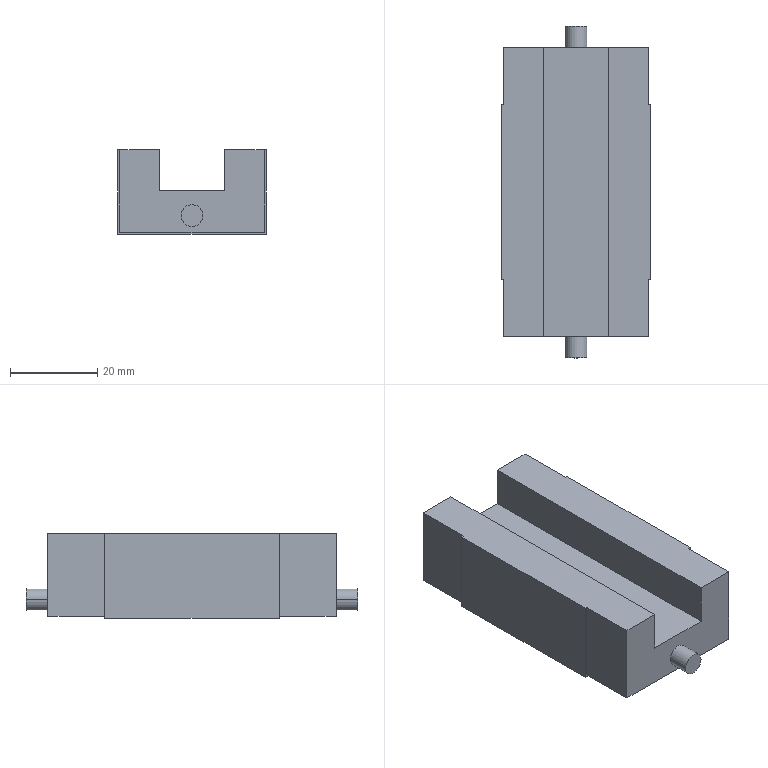Part | NX | 1 solid | 40 faces | box 34 x 76 x 19.4 mm | volume 33253 mm3 | plane 20 | cylinder 12 | cone 8 | commonest cylinder face diameters 3.3 x8 5 x4
STEP:
#1=CARTESIAN_POINT('',(33.5,0.,-18.9));
#2=VERTEX_POINT('',#1);
#3=CARTESIAN_POINT('',(33.5,0.,0.));
#4=VERTEX_POINT('',#3);
#5=CARTESIAN_POINT('',(33.5,0.,-18.9));
#6=DIRECTION('',(0.,0.,1.));
#7=VECTOR('',#6,1000.);
#8=LINE('',#5,#7);
#9=EDGE_CURVE('',#2,#4,#8,.T.);
#10=ORIENTED_EDGE('',*,*,#9,.T.);
#11=CARTESIAN_POINT('',(24.5,0.,0.));
#12=VERTEX_POINT('',#11);
#13=CARTESIAN_POINT('',(33.5,0.,0.));
#14=DIRECTION('',(-1.,0.,0.));
#15=VECTOR('',#14,1000.);
#16=LINE('',#13,#15);
#17=EDGE_CURVE('',#4,#12,#16,.T.);
#18=ORIENTED_EDGE('',*,*,#17,.T.);
#19=CARTESIAN_POINT('',(24.5,0.,-9.4));
#20=VERTEX_POINT('',#19);
#21=CARTESIAN_POINT('',(24.5,0.,0.));
#22=DIRECTION('',(0.,0.,-1.));
#23=VECTOR('',#22,1000.);
#24=LINE('',#21,#23);
#25=EDGE_CURVE('',#12,#20,#24,.T.);
#26=ORIENTED_EDGE('',*,*,#25,.T.);
#27=CARTESIAN_POINT('',(9.5,0.,-9.4));
#28=VERTEX_POINT('',#27);
#29=CARTESIAN_POINT('',(24.5,0.,-9.4));
#30=DIRECTION('',(-1.,0.,0.));
#31=VECTOR('',#30,1000.);
#32=LINE('',#29,#31);
#33=EDGE_CURVE('',#20,#28,#32,.T.);
#34=ORIENTED_EDGE('',*,*,#33,.T.);
#35=CARTESIAN_POINT('',(9.5,0.,0.));
#36=VERTEX_POINT('',#35);
#37=CARTESIAN_POINT('',(9.5,0.,-9.4));
#38=DIRECTION('',(0.,0.,1.));
#39=VECTOR('',#38,1000.);
#40=LINE('',#37,#39);
#41=EDGE_CURVE('',#28,#36,#40,.T.);
#42=ORIENTED_EDGE('',*,*,#41,.T.);
#43=CARTESIAN_POINT('',(0.5,0.,0.));
#44=VERTEX_POINT('',#43);
#45=CARTESIAN_POINT('',(9.5,0.,0.));
#46=DIRECTION('',(-1.,0.,0.));
#47=VECTOR('',#46,1000.);
#48=LINE('',#45,#47);
#49=EDGE_CURVE('',#36,#44,#48,.T.);
#50=ORIENTED_EDGE('',*,*,#49,.T.);
#51=CARTESIAN_POINT('',(0.5,0.,-18.9));
#52=VERTEX_POINT('',#51);
#53=CARTESIAN_POINT('',(0.5,0.,-18.9));
#54=DIRECTION('',(0.,0.,1.));
#55=VECTOR('',#54,1000.);
#56=LINE('',#53,#55);
#57=EDGE_CURVE('',#52,#44,#56,.T.);
#58=ORIENTED_EDGE('',*,*,#57,.F.);
#59=CARTESIAN_POINT('',(33.5,0.,-18.9));
#60=DIRECTION('',(-1.,0.,0.));
#61=VECTOR('',#60,1000.);
#62=LINE('',#59,#61);
#63=EDGE_CURVE('',#2,#52,#62,.T.);
#64=ORIENTED_EDGE('',*,*,#63,.F.);
#65=EDGE_LOOP('',(#10,#18,#26,#34,#42,#50,#58,#64));
#66=FACE_BOUND('',#65,.T.);
#67=CARTESIAN_POINT('',(19.5,0.,-15.1));
#68=VERTEX_POINT('',#67);
#69=CARTESIAN_POINT('',(14.5,0.,-15.1));
#70=VERTEX_POINT('',#69);
#71=CARTESIAN_POINT('',(17.,0.,-15.1));
#72=DIRECTION('',(0.,-1.,0.));
#73=DIRECTION('',(1.,0.,0.));
#74=AXIS2_PLACEMENT_3D('',#71,#72,#73);
#75=CIRCLE('',#74,2.5);
#76=EDGE_CURVE('',#68,#70,#75,.T.);
#77=ORIENTED_EDGE('',*,*,#76,.F.);
#78=CARTESIAN_POINT('',(17.,0.,-15.1));
#79=DIRECTION('',(0.,-1.,0.));
#80=DIRECTION('',(1.,0.,0.));
#81=AXIS2_PLACEMENT_3D('',#78,#79,#80);
#82=CIRCLE('',#81,2.5);
#83=EDGE_CURVE('',#70,#68,#82,.T.);
#84=ORIENTED_EDGE('',*,*,#83,.F.);
#85=EDGE_LOOP('',(#77,#84));
#86=FACE_BOUND('',#85,.T.);
#87=CARTESIAN_POINT('',(0.,0.,0.));
#88=DIRECTION('',(0.,1.,0.));
#89=DIRECTION('',(1.,0.,0.));
#90=AXIS2_PLACEMENT_3D('',#87,#88,#89);
#91=PLANE('',#90);
#92=ADVANCED_FACE('',(#66,#86),#91,.F.);
#93=ORIENTED_EDGE('',*,*,#9,.F.);
#94=CARTESIAN_POINT('',(33.5,13.,-18.9));
#95=VERTEX_POINT('',#94);
#96=CARTESIAN_POINT('',(33.5,0.,-18.9));
#97=DIRECTION('',(0.,1.,0.));
#98=VECTOR('',#97,1000.);
#99=LINE('',#96,#98);
#100=EDGE_CURVE('',#2,#95,#99,.T.);
#101=ORIENTED_EDGE('',*,*,#100,.T.);
#102=CARTESIAN_POINT('',(33.5,13.,0.));
#103=VERTEX_POINT('',#102);
#104=CARTESIAN_POINT('',(33.5,13.,0.));
#105=DIRECTION('',(0.,0.,-1.));
#106=VECTOR('',#105,1000.);
#107=LINE('',#104,#106);
#108=EDGE_CURVE('',#103,#95,#107,.T.);
#109=ORIENTED_EDGE('',*,*,#108,.F.);
#110=CARTESIAN_POINT('',(33.5,13.,0.));
#111=DIRECTION('',(0.,-1.,0.));
#112=VECTOR('',#111,1000.);
#113=LINE('',#110,#112);
#114=EDGE_CURVE('',#103,#4,#113,.T.);
#115=ORIENTED_EDGE('',*,*,#114,.T.);
#116=EDGE_LOOP('',(#93,#101,#109,#115));
#117=FACE_BOUND('',#116,.T.);
#118=CARTESIAN_POINT('',(33.5,0.,-18.9));
#119=DIRECTION('',(-1.,0.,0.));
#120=DIRECTION('',(0.,0.,1.));
#121=AXIS2_PLACEMENT_3D('',#118,#119,#120);
#122=PLANE('',#121);
#123=ADVANCED_FACE('',(#117),#122,.F.);
#124=CARTESIAN_POINT('',(33.5,53.,0.));
#125=VERTEX_POINT('',#124);
#126=CARTESIAN_POINT('',(34.,53.,0.));
#127=VERTEX_POINT('',#126);
#128=CARTESIAN_POINT('',(33.5,53.,0.));
#129=DIRECTION('',(1.,0.,0.));
#130=VECTOR('',#129,1000.);
#131=LINE('',#128,#130);
#132=EDGE_CURVE('',#125,#127,#131,.T.);
#133=ORIENTED_EDGE('',*,*,#132,.F.);
#134=CARTESIAN_POINT('',(33.5,66.,0.));
#135=VERTEX_POINT('',#134);
#136=CARTESIAN_POINT('',(33.5,53.,0.));
#137=DIRECTION('',(0.,1.,0.));
#138=VECTOR('',#137,1000.);
#139=LINE('',#136,#138);
#140=EDGE_CURVE('',#125,#135,#139,.T.);
#141=ORIENTED_EDGE('',*,*,#140,.T.);
#142=CARTESIAN_POINT('',(24.5,66.,0.));
#143=VERTEX_POINT('',#142);
#144=CARTESIAN_POINT('',(33.5,66.,0.));
#145=DIRECTION('',(-1.,0.,0.));
#146=VECTOR('',#145,1000.);
#147=LINE('',#144,#146);
#148=EDGE_CURVE('',#135,#143,#147,.T.);
#149=ORIENTED_EDGE('',*,*,#148,.T.);
#150=CARTESIAN_POINT('',(24.5,66.,0.));
#151=DIRECTION('',(0.,-1.,0.));
#152=VECTOR('',#151,1000.);
#153=LINE('',#150,#152);
#154=EDGE_CURVE('',#143,#12,#153,.T.);
#155=ORIENTED_EDGE('',*,*,#154,.T.);
#156=ORIENTED_EDGE('',*,*,#17,.F.);
#157=ORIENTED_EDGE('',*,*,#114,.F.);
#158=CARTESIAN_POINT('',(34.,13.,0.));
#159=VERTEX_POINT('',#158);
#160=CARTESIAN_POINT('',(33.5,13.,0.));
#161=DIRECTION('',(1.,0.,0.));
#162=VECTOR('',#161,1000.);
#163=LINE('',#160,#162);
#164=EDGE_CURVE('',#103,#159,#163,.T.);
#165=ORIENTED_EDGE('',*,*,#164,.T.);
#166=CARTESIAN_POINT('',(34.,53.,0.));
#167=DIRECTION('',(0.,-1.,0.));
#168=VECTOR('',#167,1000.);
#169=LINE('',#166,#168);
#170=EDGE_CURVE('',#127,#159,#169,.T.);
#171=ORIENTED_EDGE('',*,*,#170,.F.);
#172=EDGE_LOOP('',(#133,#141,#149,#155,#156,#157,#165,#171));
#173=FACE_BOUND('',#172,.T.);
#174=CARTESIAN_POINT('',(24.5,0.,0.));
#175=DIRECTION('',(0.,0.,1.));
#176=DIRECTION('',(1.,0.,0.));
#177=AXIS2_PLACEMENT_3D('',#174,#175,#176);
#178=PLANE('',#177);
#179=ADVANCED_FACE('',(#173),#178,.T.);
#180=CARTESIAN_POINT('',(0.5,53.,-18.9));
#181=VERTEX_POINT('',#180);
#182=CARTESIAN_POINT('',(33.5,53.,-18.9));
#183=VERTEX_POINT('',#182);
#184=CARTESIAN_POINT('',(0.5,53.,-18.9));
#185=DIRECTION('',(1.,0.,0.));
#186=VECTOR('',#185,1000.);
#187=LINE('',#184,#186);
#188=EDGE_CURVE('',#181,#183,#187,.T.);
#189=ORIENTED_EDGE('',*,*,#188,.T.);
#190=CARTESIAN_POINT('',(33.5,53.,0.));
#191=DIRECTION('',(0.,0.,-1.));
#192=VECTOR('',#191,1000.);
#193=LINE('',#190,#192);
#194=EDGE_CURVE('',#125,#183,#193,.T.);
#195=ORIENTED_EDGE('',*,*,#194,.F.);
#196=ORIENTED_EDGE('',*,*,#132,.T.);
#197=CARTESIAN_POINT('',(34.,53.,-19.4));
#198=VERTEX_POINT('',#197);
#199=CARTESIAN_POINT('',(34.,53.,0.));
#200=DIRECTION('',(0.,0.,-1.));
#201=VECTOR('',#200,1000.);
#202=LINE('',#199,#201);
#203=EDGE_CURVE('',#127,#198,#202,.T.);
#204=ORIENTED_EDGE('',*,*,#203,.T.);
#205=CARTESIAN_POINT('',(0.,53.,-19.4));
#206=VERTEX_POINT('',#205);
#207=CARTESIAN_POINT('',(0.,53.,-19.4));
#208=DIRECTION('',(1.,0.,0.));
#209=VECTOR('',#208,1000.);
#210=LINE('',#207,#209);
#211=EDGE_CURVE('',#206,#198,#210,.T.);
#212=ORIENTED_EDGE('',*,*,#211,.F.);
#213=CARTESIAN_POINT('',(0.,53.,0.));
#214=VERTEX_POINT('',#213);
#215=CARTESIAN_POINT('',(0.,53.,-19.4));
#216=DIRECTION('',(0.,0.,1.));
#217=VECTOR('',#216,1000.);
#218=LINE('',#215,#217);
#219=EDGE_CURVE('',#206,#214,#218,.T.);
#220=ORIENTED_EDGE('',*,*,#219,.T.);
#221=CARTESIAN_POINT('',(0.5,53.,0.));
#222=VERTEX_POINT('',#221);
#223=CARTESIAN_POINT('',(0.5,53.,0.));
#224=DIRECTION('',(-1.,0.,0.));
#225=VECTOR('',#224,1000.);
#226=LINE('',#223,#225);
#227=EDGE_CURVE('',#222,#214,#226,.T.);
#228=ORIENTED_EDGE('',*,*,#227,.F.);
#229=CARTESIAN_POINT('',(0.5,53.,0.));
#230=DIRECTION('',(0.,0.,-1.));
#231=VECTOR('',#230,1000.);
#232=LINE('',#229,#231);
#233=EDGE_CURVE('',#222,#181,#232,.T.);
#234=ORIENTED_EDGE('',*,*,#233,.T.);
#235=EDGE_LOOP('',(#189,#195,#196,#204,#212,#220,#228,#234));
#236=FACE_BOUND('',#235,.T.);
#237=CARTESIAN_POINT('',(34.,53.,-18.9));
#238=DIRECTION('',(0.,-1.,0.));
#239=DIRECTION('',(0.,0.,-1.));
#240=AXIS2_PLACEMENT_3D('',#237,#238,#239);
#241=PLANE('',#240);
#242=ADVANCED_FACE('',(#236),#241,.F.);
#243=CARTESIAN_POINT('',(33.5,66.,-18.9));
#244=VERTEX_POINT('',#243);
#245=CARTESIAN_POINT('',(33.5,53.,-18.9));
#246=DIRECTION('',(0.,1.,0.));
#247=VECTOR('',#246,1000.);
#248=LINE('',#245,#247);
#249=EDGE_CURVE('',#183,#244,#248,.T.);
#250=ORIENTED_EDGE('',*,*,#249,.F.);
#251=ORIENTED_EDGE('',*,*,#188,.F.);
#252=CARTESIAN_POINT('',(0.5,66.,-18.9));
#253=VERTEX_POINT('',#252);
#254=CARTESIAN_POINT('',(0.5,53.,-18.9));
#255=DIRECTION('',(0.,1.,0.));
#256=VECTOR('',#255,1000.);
#257=LINE('',#254,#256);
#258=EDGE_CURVE('',#181,#253,#257,.T.);
#259=ORIENTED_EDGE('',*,*,#258,.T.);
#260=CARTESIAN_POINT('',(33.5,66.,-18.9));
#261=DIRECTION('',(-1.,0.,0.));
#262=VECTOR('',#261,1000.);
#263=LINE('',#260,#262);
#264=EDGE_CURVE('',#244,#253,#263,.T.);
#265=ORIENTED_EDGE('',*,*,#264,.F.);
#266=EDGE_LOOP('',(#250,#251,#259,#265));
#267=FACE_BOUND('',#266,.T.);
#268=CARTESIAN_POINT('',(34.,66.,-18.9));
#269=DIRECTION('',(0.,0.,1.));
#270=DIRECTION('',(1.,0.,0.));
#271=AXIS2_PLACEMENT_3D('',#268,#269,#270);
#272=PLANE('',#271);
#273=ADVANCED_FACE('',(#267),#272,.F.);
#274=CARTESIAN_POINT('',(33.5,66.,-18.9));
#275=DIRECTION('',(0.,0.,1.));
#276=VECTOR('',#275,1000.);
#277=LINE('',#274,#276);
#278=EDGE_CURVE('',#244,#135,#277,.T.);
#279=ORIENTED_EDGE('',*,*,#278,.T.);
#280=ORIENTED_EDGE('',*,*,#140,.F.);
#281=ORIENTED_EDGE('',*,*,#194,.T.);
#282=ORIENTED_EDGE('',*,*,#249,.T.);
#283=EDGE_LOOP('',(#279,#280,#281,#282));
#284=FACE_BOUND('',#283,.T.);
#285=CARTESIAN_POINT('',(33.5,53.,-18.9));
#286=DIRECTION('',(-1.,0.,0.));
#287=DIRECTION('',(0.,0.,1.));
#288=AXIS2_PLACEMENT_3D('',#285,#286,#287);
#289=PLANE('',#288);
#290=ADVANCED_FACE('',(#284),#289,.F.);
#291=ORIENTED_EDGE('',*,*,#278,.F.);
#292=ORIENTED_EDGE('',*,*,#264,.T.);
#293=CARTESIAN_POINT('',(0.5,66.,0.));
#294=VERTEX_POINT('',#293);
#295=CARTESIAN_POINT('',(0.5,66.,-18.9));
#296=DIRECTION('',(0.,0.,1.));
#297=VECTOR('',#296,1000.);
#298=LINE('',#295,#297);
#299=EDGE_CURVE('',#253,#294,#298,.T.);
#300=ORIENTED_EDGE('',*,*,#299,.T.);
#301=CARTESIAN_POINT('',(9.5,66.,0.));
#302=VERTEX_POINT('',#301);
#303=CARTESIAN_POINT('',(9.5,66.,0.));
#304=DIRECTION('',(-1.,0.,0.));
#305=VECTOR('',#304,1000.);
#306=LINE('',#303,#305);
#307=EDGE_CURVE('',#302,#294,#306,.T.);
#308=ORIENTED_EDGE('',*,*,#307,.F.);
#309=CARTESIAN_POINT('',(9.5,66.,-9.4));
#310=VERTEX_POINT('',#309);
#311=CARTESIAN_POINT('',(9.5,66.,-9.4));
#312=DIRECTION('',(0.,0.,1.));
#313=VECTOR('',#312,1000.);
#314=LINE('',#311,#313);
#315=EDGE_CURVE('',#310,#302,#314,.T.);
#316=ORIENTED_EDGE('',*,*,#315,.F.);
#317=CARTESIAN_POINT('',(24.5,66.,-9.4));
#318=VERTEX_POINT('',#317);
#319=CARTESIAN_POINT('',(24.5,66.,-9.4));
#320=DIRECTION('',(-1.,0.,0.));
#321=VECTOR('',#320,1000.);
#322=LINE('',#319,#321);
#323=EDGE_CURVE('',#318,#310,#322,.T.);
#324=ORIENTED_EDGE('',*,*,#323,.F.);
#325=CARTESIAN_POINT('',(24.5,66.,0.));
#326=DIRECTION('',(0.,0.,-1.));
#327=VECTOR('',#326,1000.);
#328=LINE('',#325,#327);
#329=EDGE_CURVE('',#143,#318,#328,.T.);
#330=ORIENTED_EDGE('',*,*,#329,.F.);
#331=ORIENTED_EDGE('',*,*,#148,.F.);
#332=EDGE_LOOP('',(#291,#292,#300,#308,#316,#324,#330,#331));
#333=FACE_BOUND('',#332,.T.);
#334=CARTESIAN_POINT('',(19.5,66.,-15.1));
#335=VERTEX_POINT('',#334);
#336=CARTESIAN_POINT('',(14.5,66.,-15.1));
#337=VERTEX_POINT('',#336);
#338=CARTESIAN_POINT('',(17.,66.,-15.1));
#339=DIRECTION('',(0.,1.,0.));
#340=DIRECTION('',(-1.,0.,0.));
#341=AXIS2_PLACEMENT_3D('',#338,#339,#340);
#342=CIRCLE('',#341,2.5);
#343=EDGE_CURVE('',#335,#337,#342,.T.);
#344=ORIENTED_EDGE('',*,*,#343,.F.);
#345=CARTESIAN_POINT('',(17.,66.,-15.1));
#346=DIRECTION('',(0.,1.,0.));
#347=DIRECTION('',(-1.,0.,0.));
#348=AXIS2_PLACEMENT_3D('',#345,#346,#347);
#349=CIRCLE('',#348,2.5);
#350=EDGE_CURVE('',#337,#335,#349,.T.);
#351=ORIENTED_EDGE('',*,*,#350,.F.);
#352=EDGE_LOOP('',(#344,#351));
#353=FACE_BOUND('',#352,.T.);
#354=CARTESIAN_POINT('',(0.,66.,0.));
#355=DIRECTION('',(0.,1.,0.));
#356=DIRECTION('',(1.,0.,0.));
#357=AXIS2_PLACEMENT_3D('',#354,#355,#356);
#358=PLANE('',#357);
#359=ADVANCED_FACE('',(#333,#353),#358,.T.);
#360=ORIENTED_EDGE('',*,*,#25,.F.);
#361=ORIENTED_EDGE('',*,*,#154,.F.);
#362=ORIENTED_EDGE('',*,*,#329,.T.);
#363=CARTESIAN_POINT('',(24.5,66.,-9.4));
#364=DIRECTION('',(0.,-1.,0.));
#365=VECTOR('',#364,1000.);
#366=LINE('',#363,#365);
#367=EDGE_CURVE('',#318,#20,#366,.T.);
#368=ORIENTED_EDGE('',*,*,#367,.T.);
#369=EDGE_LOOP('',(#360,#361,#362,#368));
#370=FACE_BOUND('',#369,.T.);
#371=CARTESIAN_POINT('',(24.5,0.,-9.4));
#372=DIRECTION('',(-1.,0.,0.));
#373=DIRECTION('',(0.,0.,1.));
#374=AXIS2_PLACEMENT_3D('',#371,#372,#373);
#375=PLANE('',#374);
#376=ADVANCED_FACE('',(#370),#375,.T.);
#377=ORIENTED_EDGE('',*,*,#33,.F.);
#378=ORIENTED_EDGE('',*,*,#367,.F.);
#379=ORIENTED_EDGE('',*,*,#323,.T.);
#380=CARTESIAN_POINT('',(9.5,66.,-9.4));
#381=DIRECTION('',(0.,-1.,0.));
#382=VECTOR('',#381,1000.);
#383=LINE('',#380,#382);
#384=EDGE_CURVE('',#310,#28,#383,.T.);
#385=ORIENTED_EDGE('',*,*,#384,.T.);
#386=EDGE_LOOP('',(#377,#378,#379,#385));
#387=FACE_BOUND('',#386,.T.);
#388=CARTESIAN_POINT('',(9.5,0.,-9.4));
#389=DIRECTION('',(0.,0.,1.));
#390=DIRECTION('',(1.,0.,0.));
#391=AXIS2_PLACEMENT_3D('',#388,#389,#390);
#392=PLANE('',#391);
#393=ADVANCED_FACE('',(#387),#392,.T.);
#394=ORIENTED_EDGE('',*,*,#41,.F.);
#395=ORIENTED_EDGE('',*,*,#384,.F.);
#396=ORIENTED_EDGE('',*,*,#315,.T.);
#397=CARTESIAN_POINT('',(9.5,66.,0.));
#398=DIRECTION('',(0.,-1.,0.));
#399=VECTOR('',#398,1000.);
#400=LINE('',#397,#399);
#401=EDGE_CURVE('',#302,#36,#400,.T.);
#402=ORIENTED_EDGE('',*,*,#401,.T.);
#403=EDGE_LOOP('',(#394,#395,#396,#402));
#404=FACE_BOUND('',#403,.T.);
#405=CARTESIAN_POINT('',(9.5,0.,0.));
#406=DIRECTION('',(1.,0.,0.));
#407=DIRECTION('',(0.,1.,0.));
#408=AXIS2_PLACEMENT_3D('',#405,#406,#407);
#409=PLANE('',#408);
#410=ADVANCED_FACE('',(#404),#409,.T.);
#411=CARTESIAN_POINT('',(0.5,53.,0.));
#412=DIRECTION('',(0.,1.,0.));
#413=VECTOR('',#412,1000.);
#414=LINE('',#411,#413);
#415=EDGE_CURVE('',#222,#294,#414,.T.);
#416=ORIENTED_EDGE('',*,*,#415,.F.);
#417=ORIENTED_EDGE('',*,*,#227,.T.);
#418=CARTESIAN_POINT('',(0.,13.,0.));
#419=VERTEX_POINT('',#418);
#420=CARTESIAN_POINT('',(0.,53.,0.));
#421=DIRECTION('',(0.,-1.,0.));
#422=VECTOR('',#421,1000.);
#423=LINE('',#420,#422);
#424=EDGE_CURVE('',#214,#419,#423,.T.);
#425=ORIENTED_EDGE('',*,*,#424,.T.);
#426=CARTESIAN_POINT('',(0.5,13.,0.));
#427=VERTEX_POINT('',#426);
#428=CARTESIAN_POINT('',(0.5,13.,0.));
#429=DIRECTION('',(-1.,0.,0.));
#430=VECTOR('',#429,1000.);
#431=LINE('',#428,#430);
#432=EDGE_CURVE('',#427,#419,#431,.T.);
#433=ORIENTED_EDGE('',*,*,#432,.F.);
#434=CARTESIAN_POINT('',(0.5,13.,0.));
#435=DIRECTION('',(0.,-1.,0.));
#436=VECTOR('',#435,1000.);
#437=LINE('',#434,#436);
#438=EDGE_CURVE('',#427,#44,#437,.T.);
#439=ORIENTED_EDGE('',*,*,#438,.T.);
#440=ORIENTED_EDGE('',*,*,#49,.F.);
#441=ORIENTED_EDGE('',*,*,#401,.F.);
#442=ORIENTED_EDGE('',*,*,#307,.T.);
#443=EDGE_LOOP('',(#416,#417,#425,#433,#439,#440,#441,#442));
#444=FACE_BOUND('',#443,.T.);
#445=CARTESIAN_POINT('',(0.,0.,0.));
#446=DIRECTION('',(0.,0.,1.));
#447=DIRECTION('',(1.,0.,0.));
#448=AXIS2_PLACEMENT_3D('',#445,#446,#447);
#449=PLANE('',#448);
#450=ADVANCED_FACE('',(#444),#449,.T.);
#451=ORIENTED_EDGE('',*,*,#299,.F.);
#452=ORIENTED_EDGE('',*,*,#258,.F.);
#453=ORIENTED_EDGE('',*,*,#233,.F.);
#454=ORIENTED_EDGE('',*,*,#415,.T.);
#455=EDGE_LOOP('',(#451,#452,#453,#454));
#456=FACE_BOUND('',#455,.T.);
#457=CARTESIAN_POINT('',(0.5,66.,-18.9));
#458=DIRECTION('',(1.,0.,0.));
#459=DIRECTION('',(0.,1.,0.));
#460=AXIS2_PLACEMENT_3D('',#457,#458,#459);
#461=PLANE('',#460);
#462=ADVANCED_FACE('',(#456),#461,.F.);
#463=ORIENTED_EDGE('',*,*,#57,.T.);
#464=ORIENTED_EDGE('',*,*,#438,.F.);
#465=CARTESIAN_POINT('',(0.5,13.,-18.9));
#466=VERTEX_POINT('',#465);
#467=CARTESIAN_POINT('',(0.5,13.,0.));
#468=DIRECTION('',(0.,0.,-1.));
#469=VECTOR('',#468,1000.);
#470=LINE('',#467,#469);
#471=EDGE_CURVE('',#427,#466,#470,.T.);
#472=ORIENTED_EDGE('',*,*,#471,.T.);
#473=CARTESIAN_POINT('',(0.5,0.,-18.9));
#474=DIRECTION('',(0.,1.,0.));
#475=VECTOR('',#474,1000.);
#476=LINE('',#473,#475);
#477=EDGE_CURVE('',#52,#466,#476,.T.);
#478=ORIENTED_EDGE('',*,*,#477,.F.);
#479=EDGE_LOOP('',(#463,#464,#472,#478));
#480=FACE_BOUND('',#479,.T.);
#481=CARTESIAN_POINT('',(0.5,13.,-18.9));
#482=DIRECTION('',(1.,0.,0.));
#483=DIRECTION('',(0.,1.,0.));
#484=AXIS2_PLACEMENT_3D('',#481,#482,#483);
#485=PLANE('',#484);
#486=ADVANCED_FACE('',(#480),#485,.F.);
#487=ORIENTED_EDGE('',*,*,#100,.F.);
#488=ORIENTED_EDGE('',*,*,#63,.T.);
#489=ORIENTED_EDGE('',*,*,#477,.T.);
#490=CARTESIAN_POINT('',(0.5,13.,-18.9));
#491=DIRECTION('',(1.,0.,0.));
#492=VECTOR('',#491,1000.);
#493=LINE('',#490,#492);
#494=EDGE_CURVE('',#466,#95,#493,.T.);
#495=ORIENTED_EDGE('',*,*,#494,.T.);
#496=EDGE_LOOP('',(#487,#488,#489,#495));
#497=FACE_BOUND('',#496,.T.);
#498=CARTESIAN_POINT('',(34.,13.,-18.9));
#499=DIRECTION('',(0.,0.,1.));
#500=DIRECTION('',(1.,0.,0.));
#501=AXIS2_PLACEMENT_3D('',#498,#499,#500);
#502=PLANE('',#501);
#503=ADVANCED_FACE('',(#497),#502,.F.);
#504=CARTESIAN_POINT('',(0.,13.,-19.4));
#505=VERTEX_POINT('',#504);
#506=CARTESIAN_POINT('',(0.,13.,0.));
#507=DIRECTION('',(0.,0.,-1.));
#508=VECTOR('',#507,1000.);
#509=LINE('',#506,#508);
#510=EDGE_CURVE('',#419,#505,#509,.T.);
#511=ORIENTED_EDGE('',*,*,#510,.T.);
#512=CARTESIAN_POINT('',(34.,13.,-19.4));
#513=VERTEX_POINT('',#512);
#514=CARTESIAN_POINT('',(0.,13.,-19.4));
#515=DIRECTION('',(1.,0.,0.));
#516=VECTOR('',#515,1000.);
#517=LINE('',#514,#516);
#518=EDGE_CURVE('',#505,#513,#517,.T.);
#519=ORIENTED_EDGE('',*,*,#518,.T.);
#520=CARTESIAN_POINT('',(34.,13.,-19.4));
#521=DIRECTION('',(0.,0.,1.));
#522=VECTOR('',#521,1000.);
#523=LINE('',#520,#522);
#524=EDGE_CURVE('',#513,#159,#523,.T.);
#525=ORIENTED_EDGE('',*,*,#524,.T.);
#526=ORIENTED_EDGE('',*,*,#164,.F.);
#527=ORIENTED_EDGE('',*,*,#108,.T.);
#528=ORIENTED_EDGE('',*,*,#494,.F.);
#529=ORIENTED_EDGE('',*,*,#471,.F.);
#530=ORIENTED_EDGE('',*,*,#432,.T.);
#531=EDGE_LOOP('',(#511,#519,#525,#526,#527,#528,#529,#530));
#532=FACE_BOUND('',#531,.T.);
#533=CARTESIAN_POINT('',(34.,13.,-19.4));
#534=DIRECTION('',(0.,1.,0.));
#535=DIRECTION('',(1.,0.,0.));
#536=AXIS2_PLACEMENT_3D('',#533,#534,#535);
#537=PLANE('',#536);
#538=ADVANCED_FACE('',(#532),#537,.F.);
#539=ORIENTED_EDGE('',*,*,#219,.F.);
#540=CARTESIAN_POINT('',(0.,53.,-19.4));
#541=DIRECTION('',(0.,-1.,0.));
#542=VECTOR('',#541,1000.);
#543=LINE('',#540,#542);
#544=EDGE_CURVE('',#206,#505,#543,.T.);
#545=ORIENTED_EDGE('',*,*,#544,.T.);
#546=ORIENTED_EDGE('',*,*,#510,.F.);
#547=ORIENTED_EDGE('',*,*,#424,.F.);
#548=EDGE_LOOP('',(#539,#545,#546,#547));
#549=FACE_BOUND('',#548,.T.);
#550=CARTESIAN_POINT('',(0.,0.,-19.4));
#551=DIRECTION('',(-1.,0.,0.));
#552=DIRECTION('',(0.,0.,1.));
#553=AXIS2_PLACEMENT_3D('',#550,#551,#552);
#554=PLANE('',#553);
#555=ADVANCED_FACE('',(#549),#554,.T.);
#556=ORIENTED_EDGE('',*,*,#211,.T.);
#557=CARTESIAN_POINT('',(34.,53.,-19.4));
#558=DIRECTION('',(0.,-1.,0.));
#559=VECTOR('',#558,1000.);
#560=LINE('',#557,#559);
#561=EDGE_CURVE('',#198,#513,#560,.T.);
#562=ORIENTED_EDGE('',*,*,#561,.T.);
#563=ORIENTED_EDGE('',*,*,#518,.F.);
#564=ORIENTED_EDGE('',*,*,#544,.F.);
#565=EDGE_LOOP('',(#556,#562,#563,#564));
#566=FACE_BOUND('',#565,.T.);
#567=CARTESIAN_POINT('',(31.65,20.,-19.4));
#568=VERTEX_POINT('',#567);
#569=CARTESIAN_POINT('',(28.35,20.,-19.4));
#570=VERTEX_POINT('',#569);
#571=CARTESIAN_POINT('',(30.,20.,-19.4));
#572=DIRECTION('',(0.,0.,-1.));
#573=DIRECTION('',(-1.,0.,0.));
#574=AXIS2_PLACEMENT_3D('',#571,#572,#573);
#575=CIRCLE('',#574,1.65);
#576=EDGE_CURVE('',#568,#570,#575,.T.);
#577=ORIENTED_EDGE('',*,*,#576,.F.);
#578=CARTESIAN_POINT('',(30.,20.,-19.4));
#579=DIRECTION('',(0.,0.,-1.));
#580=DIRECTION('',(-1.,0.,0.));
#581=AXIS2_PLACEMENT_3D('',#578,#579,#580);
#582=CIRCLE('',#581,1.65);
#583=EDGE_CURVE('',#570,#568,#582,.T.);
#584=ORIENTED_EDGE('',*,*,#583,.F.);
#585=EDGE_LOOP('',(#577,#584));
#586=FACE_BOUND('',#585,.T.);
#587=CARTESIAN_POINT('',(28.35,46.,-19.4));
#588=VERTEX_POINT('',#587);
#589=CARTESIAN_POINT('',(31.65,46.,-19.4));
#590=VERTEX_POINT('',#589);
#591=CARTESIAN_POINT('',(30.,46.,-19.4));
#592=DIRECTION('',(0.,0.,-1.));
#593=DIRECTION('',(-1.,0.,0.));
#594=AXIS2_PLACEMENT_3D('',#591,#592,#593);
#595=CIRCLE('',#594,1.65);
#596=EDGE_CURVE('',#588,#590,#595,.T.);
#597=ORIENTED_EDGE('',*,*,#596,.F.);
#598=CARTESIAN_POINT('',(30.,46.,-19.4));
#599=DIRECTION('',(0.,0.,-1.));
#600=DIRECTION('',(-1.,0.,0.));
#601=AXIS2_PLACEMENT_3D('',#598,#599,#600);
#602=CIRCLE('',#601,1.65);
#603=EDGE_CURVE('',#590,#588,#602,.T.);
#604=ORIENTED_EDGE('',*,*,#603,.F.);
#605=EDGE_LOOP('',(#597,#604));
#606=FACE_BOUND('',#605,.T.);
#607=CARTESIAN_POINT('',(2.35,20.,-19.4));
#608=VERTEX_POINT('',#607);
#609=CARTESIAN_POINT('',(5.65,20.,-19.4));
#610=VERTEX_POINT('',#609);
#611=CARTESIAN_POINT('',(4.,20.,-19.4));
#612=DIRECTION('',(0.,0.,-1.));
#613=DIRECTION('',(-1.,0.,0.));
#614=AXIS2_PLACEMENT_3D('',#611,#612,#613);
#615=CIRCLE('',#614,1.65);
#616=EDGE_CURVE('',#608,#610,#615,.T.);
#617=ORIENTED_EDGE('',*,*,#616,.F.);
#618=CARTESIAN_POINT('',(4.,20.,-19.4));
#619=DIRECTION('',(0.,0.,-1.));
#620=DIRECTION('',(-1.,0.,0.));
#621=AXIS2_PLACEMENT_3D('',#618,#619,#620);
#622=CIRCLE('',#621,1.65);
#623=EDGE_CURVE('',#610,#608,#622,.T.);
#624=ORIENTED_EDGE('',*,*,#623,.F.);
#625=EDGE_LOOP('',(#617,#624));
#626=FACE_BOUND('',#625,.T.);
#627=CARTESIAN_POINT('',(5.65,46.,-19.4));
#628=VERTEX_POINT('',#627);
#629=CARTESIAN_POINT('',(2.35,46.,-19.4));
#630=VERTEX_POINT('',#629);
#631=CARTESIAN_POINT('',(4.,46.,-19.4));
#632=DIRECTION('',(0.,0.,-1.));
#633=DIRECTION('',(-1.,0.,0.));
#634=AXIS2_PLACEMENT_3D('',#631,#632,#633);
#635=CIRCLE('',#634,1.65);
#636=EDGE_CURVE('',#628,#630,#635,.T.);
#637=ORIENTED_EDGE('',*,*,#636,.F.);
#638=CARTESIAN_POINT('',(4.,46.,-19.4));
#639=DIRECTION('',(0.,0.,-1.));
#640=DIRECTION('',(-1.,0.,0.));
#641=AXIS2_PLACEMENT_3D('',#638,#639,#640);
#642=CIRCLE('',#641,1.65);
#643=EDGE_CURVE('',#630,#628,#642,.T.);
#644=ORIENTED_EDGE('',*,*,#643,.F.);
#645=EDGE_LOOP('',(#637,#644));
#646=FACE_BOUND('',#645,.T.);
#647=CARTESIAN_POINT('',(34.,0.,-19.4));
#648=DIRECTION('',(0.,0.,-1.));
#649=DIRECTION('',(0.,-1.,0.));
#650=AXIS2_PLACEMENT_3D('',#647,#648,#649);
#651=PLANE('',#650);
#652=ADVANCED_FACE('',(#566,#586,#606,#626,#646),#651,.T.);
#653=ORIENTED_EDGE('',*,*,#203,.F.);
#654=ORIENTED_EDGE('',*,*,#170,.T.);
#655=ORIENTED_EDGE('',*,*,#524,.F.);
#656=ORIENTED_EDGE('',*,*,#561,.F.);
#657=EDGE_LOOP('',(#653,#654,#655,#656));
#658=FACE_BOUND('',#657,.T.);
#659=CARTESIAN_POINT('',(34.,0.,0.));
#660=DIRECTION('',(1.,0.,0.));
#661=DIRECTION('',(0.,1.,0.));
#662=AXIS2_PLACEMENT_3D('',#659,#660,#661);
#663=PLANE('',#662);
#664=ADVANCED_FACE('',(#658),#663,.T.);
#665=ORIENTED_EDGE('',*,*,#576,.T.);
#666=CARTESIAN_POINT('',(28.35,20.,-12.8));
#667=VERTEX_POINT('',#666);
#668=CARTESIAN_POINT('',(28.35,20.,-11.429));
#669=DIRECTION('',(0.,0.,-1.));
#670=VECTOR('',#669,1000.);
#671=LINE('',#668,#670);
#672=EDGE_CURVE('',#667,#570,#671,.T.);
#673=ORIENTED_EDGE('',*,*,#672,.F.);
#674=CARTESIAN_POINT('',(31.65,20.,-12.8));
#675=VERTEX_POINT('',#674);
#676=CARTESIAN_POINT('',(30.,20.,-12.8));
#677=DIRECTION('',(0.,0.,1.));
#678=DIRECTION('',(-1.,0.,0.));
#679=AXIS2_PLACEMENT_3D('',#676,#677,#678);
#680=CIRCLE('',#679,1.65);
#681=EDGE_CURVE('',#667,#675,#680,.T.);
#682=ORIENTED_EDGE('',*,*,#681,.T.);
#683=CARTESIAN_POINT('',(31.65,20.,-11.429));
#684=DIRECTION('',(0.,0.,-1.));
#685=VECTOR('',#684,1000.);
#686=LINE('',#683,#685);
#687=EDGE_CURVE('',#675,#568,#686,.T.);
#688=ORIENTED_EDGE('',*,*,#687,.T.);
#689=EDGE_LOOP('',(#665,#673,#682,#688));
#690=FACE_BOUND('',#689,.T.);
#691=CARTESIAN_POINT('',(30.,20.,-11.429));
#692=DIRECTION('',(0.,0.,-1.));
#693=DIRECTION('',(1.,0.,0.));
#694=AXIS2_PLACEMENT_3D('',#691,#692,#693);
#695=CYLINDRICAL_SURFACE('',#694,1.65);
#696=ADVANCED_FACE('',(#690),#695,.F.);
#697=CARTESIAN_POINT('',(5.65,46.,-12.8));
#698=VERTEX_POINT('',#697);
#699=CARTESIAN_POINT('',(2.35,46.,-12.8));
#700=VERTEX_POINT('',#699);
#701=CARTESIAN_POINT('',(4.,46.,-12.8));
#702=DIRECTION('',(0.,0.,1.));
#703=DIRECTION('',(1.,0.,0.));
#704=AXIS2_PLACEMENT_3D('',#701,#702,#703);
#705=CIRCLE('',#704,1.65);
#706=EDGE_CURVE('',#698,#700,#705,.T.);
#707=ORIENTED_EDGE('',*,*,#706,.F.);
#708=CARTESIAN_POINT('',(4.,46.,-11.809));
#709=VERTEX_POINT('',#708);
#710=CARTESIAN_POINT('',(4.869,46.,-12.331));
#711=DIRECTION('',(0.8572,0.,-0.515));
#712=VECTOR('',#711,1000.);
#713=LINE('',#710,#712);
#714=EDGE_CURVE('',#709,#698,#713,.T.);
#715=ORIENTED_EDGE('',*,*,#714,.F.);
#716=CARTESIAN_POINT('',(3.131,46.,-12.331));
#717=DIRECTION('',(-0.8572,0.,-0.515));
#718=VECTOR('',#717,1000.);
#719=LINE('',#716,#718);
#720=EDGE_CURVE('',#709,#700,#719,.T.);
#721=ORIENTED_EDGE('',*,*,#720,.T.);
#722=EDGE_LOOP('',(#707,#715,#721));
#723=FACE_BOUND('',#722,.T.);
#724=CARTESIAN_POINT('',(4.,46.,-12.331));
#725=DIRECTION('',(0.,0.,-1.));
#726=DIRECTION('',(-1.,0.,0.));
#727=AXIS2_PLACEMENT_3D('',#724,#725,#726);
#728=CONICAL_SURFACE('',#727,0.869,1.03);
#729=ADVANCED_FACE('',(#723),#728,.F.);
#730=ORIENTED_EDGE('',*,*,#681,.F.);
#731=CARTESIAN_POINT('',(30.,20.,-11.809));
#732=VERTEX_POINT('',#731);
#733=CARTESIAN_POINT('',(29.131,20.,-12.331));
#734=DIRECTION('',(-0.8572,0.,-0.515));
#735=VECTOR('',#734,1000.);
#736=LINE('',#733,#735);
#737=EDGE_CURVE('',#732,#667,#736,.T.);
#738=ORIENTED_EDGE('',*,*,#737,.F.);
#739=CARTESIAN_POINT('',(30.869,20.,-12.331));
#740=DIRECTION('',(0.8572,0.,-0.515));
#741=VECTOR('',#740,1000.);
#742=LINE('',#739,#741);
#743=EDGE_CURVE('',#732,#675,#742,.T.);
#744=ORIENTED_EDGE('',*,*,#743,.T.);
#745=EDGE_LOOP('',(#730,#738,#744));
#746=FACE_BOUND('',#745,.T.);
#747=CARTESIAN_POINT('',(30.,20.,-12.331));
#748=DIRECTION('',(0.,0.,-1.));
#749=DIRECTION('',(-1.,0.,0.));
#750=AXIS2_PLACEMENT_3D('',#747,#748,#749);
#751=CONICAL_SURFACE('',#750,0.869,1.03);
#752=ADVANCED_FACE('',(#746),#751,.F.);
#753=CARTESIAN_POINT('',(19.5,-5.,-15.1));
#754=VERTEX_POINT('',#753);
#755=CARTESIAN_POINT('',(14.5,-5.,-15.1));
#756=VERTEX_POINT('',#755);
#757=CARTESIAN_POINT('',(17.,-5.,-15.1));
#758=DIRECTION('',(0.,1.,0.));
#759=DIRECTION('',(1.,0.,0.));
#760=AXIS2_PLACEMENT_3D('',#757,#758,#759);
#761=CIRCLE('',#760,2.5);
#762=EDGE_CURVE('',#754,#756,#761,.T.);
#763=ORIENTED_EDGE('',*,*,#762,.F.);
#764=CARTESIAN_POINT('',(17.,-5.,-15.1));
#765=DIRECTION('',(0.,1.,0.));
#766=DIRECTION('',(1.,0.,0.));
#767=AXIS2_PLACEMENT_3D('',#764,#765,#766);
#768=CIRCLE('',#767,2.5);
#769=EDGE_CURVE('',#756,#754,#768,.T.);
#770=ORIENTED_EDGE('',*,*,#769,.F.);
#771=EDGE_LOOP('',(#763,#770));
#772=FACE_BOUND('',#771,.T.);
#773=CARTESIAN_POINT('',(0.,-5.,0.));
#774=DIRECTION('',(0.,-1.,0.));
#775=DIRECTION('',(0.,0.,-1.));
#776=AXIS2_PLACEMENT_3D('',#773,#774,#775);
#777=PLANE('',#776);
#778=ADVANCED_FACE('',(#772),#777,.T.);
#779=CARTESIAN_POINT('',(28.35,46.,-12.8));
#780=VERTEX_POINT('',#779);
#781=CARTESIAN_POINT('',(31.65,46.,-12.8));
#782=VERTEX_POINT('',#781);
#783=CARTESIAN_POINT('',(30.,46.,-12.8));
#784=DIRECTION('',(0.,0.,1.));
#785=DIRECTION('',(-1.,0.,0.));
#786=AXIS2_PLACEMENT_3D('',#783,#784,#785);
#787=CIRCLE('',#786,1.65);
#788=EDGE_CURVE('',#780,#782,#787,.T.);
#789=ORIENTED_EDGE('',*,*,#788,.T.);
#790=CARTESIAN_POINT('',(31.65,46.,-11.429));
#791=DIRECTION('',(0.,0.,-1.));
#792=VECTOR('',#791,1000.);
#793=LINE('',#790,#792);
#794=EDGE_CURVE('',#782,#590,#793,.T.);
#795=ORIENTED_EDGE('',*,*,#794,.T.);
#796=ORIENTED_EDGE('',*,*,#603,.T.);
#797=CARTESIAN_POINT('',(28.35,46.,-11.429));
#798=DIRECTION('',(0.,0.,-1.));
#799=VECTOR('',#798,1000.);
#800=LINE('',#797,#799);
#801=EDGE_CURVE('',#780,#588,#800,.T.);
#802=ORIENTED_EDGE('',*,*,#801,.F.);
#803=EDGE_LOOP('',(#789,#795,#796,#802));
#804=FACE_BOUND('',#803,.T.);
#805=CARTESIAN_POINT('',(30.,46.,-11.429));
#806=DIRECTION('',(0.,0.,-1.));
#807=DIRECTION('',(1.,0.,0.));
#808=AXIS2_PLACEMENT_3D('',#805,#806,#807);
#809=CYLINDRICAL_SURFACE('',#808,1.65);
#810=ADVANCED_FACE('',(#804),#809,.F.);
#811=ORIENTED_EDGE('',*,*,#76,.T.);
#812=CARTESIAN_POINT('',(14.5,0.,-15.1));
#813=DIRECTION('',(0.,-1.,0.));
#814=VECTOR('',#813,1000.);
#815=LINE('',#812,#814);
#816=EDGE_CURVE('',#756,#70,#815,.F.);
#817=ORIENTED_EDGE('',*,*,#816,.F.);
#818=ORIENTED_EDGE('',*,*,#769,.T.);
#819=CARTESIAN_POINT('',(19.5,0.,-15.1));
#820=DIRECTION('',(0.,-1.,0.));
#821=VECTOR('',#820,1000.);
#822=LINE('',#819,#821);
#823=EDGE_CURVE('',#754,#68,#822,.F.);
#824=ORIENTED_EDGE('',*,*,#823,.T.);
#825=EDGE_LOOP('',(#811,#817,#818,#824));
#826=FACE_BOUND('',#825,.T.);
#827=CARTESIAN_POINT('',(17.,0.,-15.1));
#828=DIRECTION('',(0.,-1.,0.));
#829=DIRECTION('',(-1.,0.,0.));
#830=AXIS2_PLACEMENT_3D('',#827,#828,#829);
#831=CYLINDRICAL_SURFACE('',#830,2.5);
#832=ADVANCED_FACE('',(#826),#831,.T.);
#833=ORIENTED_EDGE('',*,*,#788,.F.);
#834=CARTESIAN_POINT('',(30.,46.,-11.809));
#835=VERTEX_POINT('',#834);
#836=CARTESIAN_POINT('',(29.131,46.,-12.331));
#837=DIRECTION('',(-0.8572,0.,-0.515));
#838=VECTOR('',#837,1000.);
#839=LINE('',#836,#838);
#840=EDGE_CURVE('',#835,#780,#839,.T.);
#841=ORIENTED_EDGE('',*,*,#840,.F.);
#842=CARTESIAN_POINT('',(30.869,46.,-12.331));
#843=DIRECTION('',(0.8572,0.,-0.515));
#844=VECTOR('',#843,1000.);
#845=LINE('',#842,#844);
#846=EDGE_CURVE('',#835,#782,#845,.T.);
#847=ORIENTED_EDGE('',*,*,#846,.T.);
#848=EDGE_LOOP('',(#833,#841,#847));
#849=FACE_BOUND('',#848,.T.);
#850=CARTESIAN_POINT('',(30.,46.,-12.331));
#851=DIRECTION('',(0.,0.,-1.));
#852=DIRECTION('',(-1.,0.,0.));
#853=AXIS2_PLACEMENT_3D('',#850,#851,#852);
#854=CONICAL_SURFACE('',#853,0.869,1.03);
#855=ADVANCED_FACE('',(#849),#854,.F.);
#856=CARTESIAN_POINT('',(19.5,71.,-15.1));
#857=VERTEX_POINT('',#856);
#858=CARTESIAN_POINT('',(14.5,71.,-15.1));
#859=VERTEX_POINT('',#858);
#860=CARTESIAN_POINT('',(17.,71.,-15.1));
#861=DIRECTION('',(0.,-1.,0.));
#862=DIRECTION('',(1.,0.,0.));
#863=AXIS2_PLACEMENT_3D('',#860,#861,#862);
#864=CIRCLE('',#863,2.5);
#865=EDGE_CURVE('',#857,#859,#864,.T.);
#866=ORIENTED_EDGE('',*,*,#865,.T.);
#867=CARTESIAN_POINT('',(14.5,66.,-15.1));
#868=DIRECTION('',(0.,1.,0.));
#869=VECTOR('',#868,1000.);
#870=LINE('',#867,#869);
#871=EDGE_CURVE('',#859,#337,#870,.F.);
#872=ORIENTED_EDGE('',*,*,#871,.T.);
#873=ORIENTED_EDGE('',*,*,#350,.T.);
#874=CARTESIAN_POINT('',(19.5,66.,-15.1));
#875=DIRECTION('',(0.,1.,0.));
#876=VECTOR('',#875,1000.);
#877=LINE('',#874,#876);
#878=EDGE_CURVE('',#857,#335,#877,.F.);
#879=ORIENTED_EDGE('',*,*,#878,.F.);
#880=EDGE_LOOP('',(#866,#872,#873,#879));
#881=FACE_BOUND('',#880,.T.);
#882=CARTESIAN_POINT('',(17.,66.,-15.1));
#883=DIRECTION('',(0.,1.,0.));
#884=DIRECTION('',(1.,0.,0.));
#885=AXIS2_PLACEMENT_3D('',#882,#883,#884);
#886=CYLINDRICAL_SURFACE('',#885,2.5);
#887=ADVANCED_FACE('',(#881),#886,.T.);
#888=ORIENTED_EDGE('',*,*,#616,.T.);
#889=CARTESIAN_POINT('',(5.65,20.,-12.8));
#890=VERTEX_POINT('',#889);
#891=CARTESIAN_POINT('',(5.65,20.,-11.429));
#892=DIRECTION('',(0.,0.,-1.));
#893=VECTOR('',#892,1000.);
#894=LINE('',#891,#893);
#895=EDGE_CURVE('',#890,#610,#894,.T.);
#896=ORIENTED_EDGE('',*,*,#895,.F.);
#897=CARTESIAN_POINT('',(2.35,20.,-12.8));
#898=VERTEX_POINT('',#897);
#899=CARTESIAN_POINT('',(4.,20.,-12.8));
#900=DIRECTION('',(0.,0.,1.));
#901=DIRECTION('',(-1.,0.,0.));
#902=AXIS2_PLACEMENT_3D('',#899,#900,#901);
#903=CIRCLE('',#902,1.65);
#904=EDGE_CURVE('',#890,#898,#903,.T.);
#905=ORIENTED_EDGE('',*,*,#904,.T.);
#906=CARTESIAN_POINT('',(2.35,20.,-11.429));
#907=DIRECTION('',(0.,0.,-1.));
#908=VECTOR('',#907,1000.);
#909=LINE('',#906,#908);
#910=EDGE_CURVE('',#898,#608,#909,.T.);
#911=ORIENTED_EDGE('',*,*,#910,.T.);
#912=EDGE_LOOP('',(#888,#896,#905,#911));
#913=FACE_BOUND('',#912,.T.);
#914=CARTESIAN_POINT('',(4.,20.,-11.429));
#915=DIRECTION('',(0.,0.,-1.));
#916=DIRECTION('',(1.,0.,0.));
#917=AXIS2_PLACEMENT_3D('',#914,#915,#916);
#918=CYLINDRICAL_SURFACE('',#917,1.65);
#919=ADVANCED_FACE('',(#913),#918,.F.);
#920=ORIENTED_EDGE('',*,*,#636,.T.);
#921=CARTESIAN_POINT('',(2.35,46.,-11.429));
#922=DIRECTION('',(0.,0.,-1.));
#923=VECTOR('',#922,1000.);
#924=LINE('',#921,#923);
#925=EDGE_CURVE('',#630,#700,#924,.F.);
#926=ORIENTED_EDGE('',*,*,#925,.T.);
#927=CARTESIAN_POINT('',(4.,46.,-12.8));
#928=DIRECTION('',(0.,0.,1.));
#929=DIRECTION('',(1.,0.,0.));
#930=AXIS2_PLACEMENT_3D('',#927,#928,#929);
#931=CIRCLE('',#930,1.65);
#932=EDGE_CURVE('',#700,#698,#931,.T.);
#933=ORIENTED_EDGE('',*,*,#932,.T.);
#934=CARTESIAN_POINT('',(5.65,46.,-11.429));
#935=DIRECTION('',(0.,0.,-1.));
#936=VECTOR('',#935,1000.);
#937=LINE('',#934,#936);
#938=EDGE_CURVE('',#628,#698,#937,.F.);
#939=ORIENTED_EDGE('',*,*,#938,.F.);
#940=EDGE_LOOP('',(#920,#926,#933,#939));
#941=FACE_BOUND('',#940,.T.);
#942=CARTESIAN_POINT('',(4.,46.,-11.429));
#943=DIRECTION('',(0.,0.,-1.));
#944=DIRECTION('',(1.,0.,0.));
#945=AXIS2_PLACEMENT_3D('',#942,#943,#944);
#946=CYLINDRICAL_SURFACE('',#945,1.65);
#947=ADVANCED_FACE('',(#941),#946,.F.);
#948=CARTESIAN_POINT('',(4.,20.,-12.8));
#949=DIRECTION('',(0.,0.,1.));
#950=DIRECTION('',(-1.,0.,0.));
#951=AXIS2_PLACEMENT_3D('',#948,#949,#950);
#952=CIRCLE('',#951,1.65);
#953=EDGE_CURVE('',#898,#890,#952,.T.);
#954=ORIENTED_EDGE('',*,*,#953,.F.);
#955=CARTESIAN_POINT('',(4.,20.,-11.809));
#956=VERTEX_POINT('',#955);
#957=CARTESIAN_POINT('',(3.131,20.,-12.331));
#958=DIRECTION('',(-0.8572,0.,-0.515));
#959=VECTOR('',#958,1000.);
#960=LINE('',#957,#959);
#961=EDGE_CURVE('',#956,#898,#960,.T.);
#962=ORIENTED_EDGE('',*,*,#961,.F.);
#963=CARTESIAN_POINT('',(4.869,20.,-12.331));
#964=DIRECTION('',(0.8572,0.,-0.515));
#965=VECTOR('',#964,1000.);
#966=LINE('',#963,#965);
#967=EDGE_CURVE('',#956,#890,#966,.T.);
#968=ORIENTED_EDGE('',*,*,#967,.T.);
#969=EDGE_LOOP('',(#954,#962,#968));
#970=FACE_BOUND('',#969,.T.);
#971=CARTESIAN_POINT('',(4.,20.,-12.331));
#972=DIRECTION('',(0.,0.,-1.));
#973=DIRECTION('',(-1.,0.,0.));
#974=AXIS2_PLACEMENT_3D('',#971,#972,#973);
#975=CONICAL_SURFACE('',#974,0.869,1.03);
#976=ADVANCED_FACE('',(#970),#975,.F.);
#977=ORIENTED_EDGE('',*,*,#865,.F.);
#978=CARTESIAN_POINT('',(17.,71.,-15.1));
#979=DIRECTION('',(0.,-1.,0.));
#980=DIRECTION('',(1.,0.,0.));
#981=AXIS2_PLACEMENT_3D('',#978,#979,#980);
#982=CIRCLE('',#981,2.5);
#983=EDGE_CURVE('',#859,#857,#982,.T.);
#984=ORIENTED_EDGE('',*,*,#983,.F.);
#985=EDGE_LOOP('',(#977,#984));
#986=FACE_BOUND('',#985,.T.);
#987=CARTESIAN_POINT('',(0.,71.,0.));
#988=DIRECTION('',(0.,1.,0.));
#989=DIRECTION('',(1.,0.,0.));
#990=AXIS2_PLACEMENT_3D('',#987,#988,#989);
#991=PLANE('',#990);
#992=ADVANCED_FACE('',(#986),#991,.T.);
#993=ORIENTED_EDGE('',*,*,#706,.T.);
#994=ORIENTED_EDGE('',*,*,#925,.F.);
#995=ORIENTED_EDGE('',*,*,#643,.T.);
#996=ORIENTED_EDGE('',*,*,#938,.T.);
#997=EDGE_LOOP('',(#993,#994,#995,#996));
#998=FACE_BOUND('',#997,.T.);
#999=CARTESIAN_POINT('',(4.,46.,-11.429));
#1000=DIRECTION('',(0.,0.,-1.));
#1001=DIRECTION('',(1.,0.,0.));
#1002=AXIS2_PLACEMENT_3D('',#999,#1000,#1001);
#1003=CYLINDRICAL_SURFACE('',#1002,1.65);
#1004=ADVANCED_FACE('',(#998),#1003,.F.);
#1005=ORIENTED_EDGE('',*,*,#846,.F.);
#1006=ORIENTED_EDGE('',*,*,#840,.T.);
#1007=CARTESIAN_POINT('',(30.,46.,-12.8));
#1008=DIRECTION('',(0.,0.,1.));
#1009=DIRECTION('',(-1.,0.,0.));
#1010=AXIS2_PLACEMENT_3D('',#1007,#1008,#1009);
#1011=CIRCLE('',#1010,1.65);
#1012=EDGE_CURVE('',#782,#780,#1011,.T.);
#1013=ORIENTED_EDGE('',*,*,#1012,.F.);
#1014=EDGE_LOOP('',(#1005,#1006,#1013));
#1015=FACE_BOUND('',#1014,.T.);
#1016=CARTESIAN_POINT('',(30.,46.,-12.331));
#1017=DIRECTION('',(0.,0.,-1.));
#1018=DIRECTION('',(-1.,0.,0.));
#1019=AXIS2_PLACEMENT_3D('',#1016,#1017,#1018);
#1020=CONICAL_SURFACE('',#1019,0.869,1.03);
#1021=ADVANCED_FACE('',(#1015),#1020,.F.);
#1022=ORIENTED_EDGE('',*,*,#687,.F.);
#1023=CARTESIAN_POINT('',(30.,20.,-12.8));
#1024=DIRECTION('',(0.,0.,1.));
#1025=DIRECTION('',(-1.,0.,0.));
#1026=AXIS2_PLACEMENT_3D('',#1023,#1024,#1025);
#1027=CIRCLE('',#1026,1.65);
#1028=EDGE_CURVE('',#675,#667,#1027,.T.);
#1029=ORIENTED_EDGE('',*,*,#1028,.T.);
#1030=ORIENTED_EDGE('',*,*,#672,.T.);
#1031=ORIENTED_EDGE('',*,*,#583,.T.);
#1032=EDGE_LOOP('',(#1022,#1029,#1030,#1031));
#1033=FACE_BOUND('',#1032,.T.);
#1034=CARTESIAN_POINT('',(30.,20.,-11.429));
#1035=DIRECTION('',(0.,0.,-1.));
#1036=DIRECTION('',(1.,0.,0.));
#1037=AXIS2_PLACEMENT_3D('',#1034,#1035,#1036);
#1038=CYLINDRICAL_SURFACE('',#1037,1.65);
#1039=ADVANCED_FACE('',(#1033),#1038,.F.);
#1040=ORIENTED_EDGE('',*,*,#343,.T.);
#1041=ORIENTED_EDGE('',*,*,#871,.F.);
#1042=ORIENTED_EDGE('',*,*,#983,.T.);
#1043=ORIENTED_EDGE('',*,*,#878,.T.);
#1044=EDGE_LOOP('',(#1040,#1041,#1042,#1043));
#1045=FACE_BOUND('',#1044,.T.);
#1046=CARTESIAN_POINT('',(17.,66.,-15.1));
#1047=DIRECTION('',(0.,1.,0.));
#1048=DIRECTION('',(1.,0.,0.));
#1049=AXIS2_PLACEMENT_3D('',#1046,#1047,#1048);
#1050=CYLINDRICAL_SURFACE('',#1049,2.5);
#1051=ADVANCED_FACE('',(#1045),#1050,.T.);
#1052=ORIENTED_EDGE('',*,*,#714,.T.);
#1053=ORIENTED_EDGE('',*,*,#932,.F.);
#1054=ORIENTED_EDGE('',*,*,#720,.F.);
#1055=EDGE_LOOP('',(#1052,#1053,#1054));
#1056=FACE_BOUND('',#1055,.T.);
#1057=CARTESIAN_POINT('',(4.,46.,-12.331));
#1058=DIRECTION('',(0.,0.,-1.));
#1059=DIRECTION('',(-1.,0.,0.));
#1060=AXIS2_PLACEMENT_3D('',#1057,#1058,#1059);
#1061=CONICAL_SURFACE('',#1060,0.869,1.03);
#1062=ADVANCED_FACE('',(#1056),#1061,.F.);
#1063=ORIENTED_EDGE('',*,*,#953,.T.);
#1064=ORIENTED_EDGE('',*,*,#895,.T.);
#1065=ORIENTED_EDGE('',*,*,#623,.T.);
#1066=ORIENTED_EDGE('',*,*,#910,.F.);
#1067=EDGE_LOOP('',(#1063,#1064,#1065,#1066));
#1068=FACE_BOUND('',#1067,.T.);
#1069=CARTESIAN_POINT('',(4.,20.,-11.429));
#1070=DIRECTION('',(0.,0.,-1.));
#1071=DIRECTION('',(1.,0.,0.));
#1072=AXIS2_PLACEMENT_3D('',#1069,#1070,#1071);
#1073=CYLINDRICAL_SURFACE('',#1072,1.65);
#1074=ADVANCED_FACE('',(#1068),#1073,.F.);
#1075=ORIENTED_EDGE('',*,*,#743,.F.);
#1076=ORIENTED_EDGE('',*,*,#737,.T.);
#1077=ORIENTED_EDGE('',*,*,#1028,.F.);
#1078=EDGE_LOOP('',(#1075,#1076,#1077));
#1079=FACE_BOUND('',#1078,.T.);
#1080=CARTESIAN_POINT('',(30.,20.,-12.331));
#1081=DIRECTION('',(0.,0.,-1.));
#1082=DIRECTION('',(-1.,0.,0.));
#1083=AXIS2_PLACEMENT_3D('',#1080,#1081,#1082);
#1084=CONICAL_SURFACE('',#1083,0.869,1.03);
#1085=ADVANCED_FACE('',(#1079),#1084,.F.);
#1086=ORIENTED_EDGE('',*,*,#762,.T.);
#1087=ORIENTED_EDGE('',*,*,#816,.T.);
#1088=ORIENTED_EDGE('',*,*,#83,.T.);
#1089=ORIENTED_EDGE('',*,*,#823,.F.);
#1090=EDGE_LOOP('',(#1086,#1087,#1088,#1089));
#1091=FACE_BOUND('',#1090,.T.);
#1092=CARTESIAN_POINT('',(17.,0.,-15.1));
#1093=DIRECTION('',(0.,-1.,0.));
#1094=DIRECTION('',(-1.,0.,0.));
#1095=AXIS2_PLACEMENT_3D('',#1092,#1093,#1094);
#1096=CYLINDRICAL_SURFACE('',#1095,2.5);
#1097=ADVANCED_FACE('',(#1091),#1096,.T.);
#1098=ORIENTED_EDGE('',*,*,#967,.F.);
#1099=ORIENTED_EDGE('',*,*,#961,.T.);
#1100=ORIENTED_EDGE('',*,*,#904,.F.);
#1101=EDGE_LOOP('',(#1098,#1099,#1100));
#1102=FACE_BOUND('',#1101,.T.);
#1103=CARTESIAN_POINT('',(4.,20.,-12.331));
#1104=DIRECTION('',(0.,0.,-1.));
#1105=DIRECTION('',(-1.,0.,0.));
#1106=AXIS2_PLACEMENT_3D('',#1103,#1104,#1105);
#1107=CONICAL_SURFACE('',#1106,0.869,1.03);
#1108=ADVANCED_FACE('',(#1102),#1107,.F.);
#1109=ORIENTED_EDGE('',*,*,#596,.T.);
#1110=ORIENTED_EDGE('',*,*,#794,.F.);
#1111=ORIENTED_EDGE('',*,*,#1012,.T.);
#1112=ORIENTED_EDGE('',*,*,#801,.T.);
#1113=EDGE_LOOP('',(#1109,#1110,#1111,#1112));
#1114=FACE_BOUND('',#1113,.T.);
#1115=CARTESIAN_POINT('',(30.,46.,-11.429));
#1116=DIRECTION('',(0.,0.,-1.));
#1117=DIRECTION('',(1.,0.,0.));
#1118=AXIS2_PLACEMENT_3D('',#1115,#1116,#1117);
#1119=CYLINDRICAL_SURFACE('',#1118,1.65);
#1120=ADVANCED_FACE('',(#1114),#1119,.F.);
#1121=CLOSED_SHELL('',(#92,#123,#179,#242,#273,#290,#359,#376,#393,#410,#450,#462,#486,#503,#538,#555,#652,#664,#696,#729,#752,#778,#810,#832,#855,#887,#919,#947,#976,#992,#1004,#1021,#1039,#1051,#1062,#1074,#1085,#1097,#1108,#1120));
#1122=MANIFOLD_SOLID_BREP('',#1121);
#1123=(LENGTH_UNIT()NAMED_UNIT(*)SI_UNIT(.MILLI.,.METRE.));
#1124=UNCERTAINTY_MEASURE_WITH_UNIT(LENGTH_MEASURE(0.00001),#1123,'','');
#1125=(NAMED_UNIT(*)PLANE_ANGLE_UNIT()SI_UNIT($,.RADIAN.));
#1126=(NAMED_UNIT(*)SI_UNIT($,.STERADIAN.)SOLID_ANGLE_UNIT());
#1127=(GEOMETRIC_REPRESENTATION_CONTEXT(3)GLOBAL_UNCERTAINTY_ASSIGNED_CONTEXT((#1124))GLOBAL_UNIT_ASSIGNED_CONTEXT((#1123,#1125,#1126))REPRESENTATION_CONTEXT('',''));
#1128=ADVANCED_BREP_SHAPE_REPRESENTATION('',(#1122),#1127);